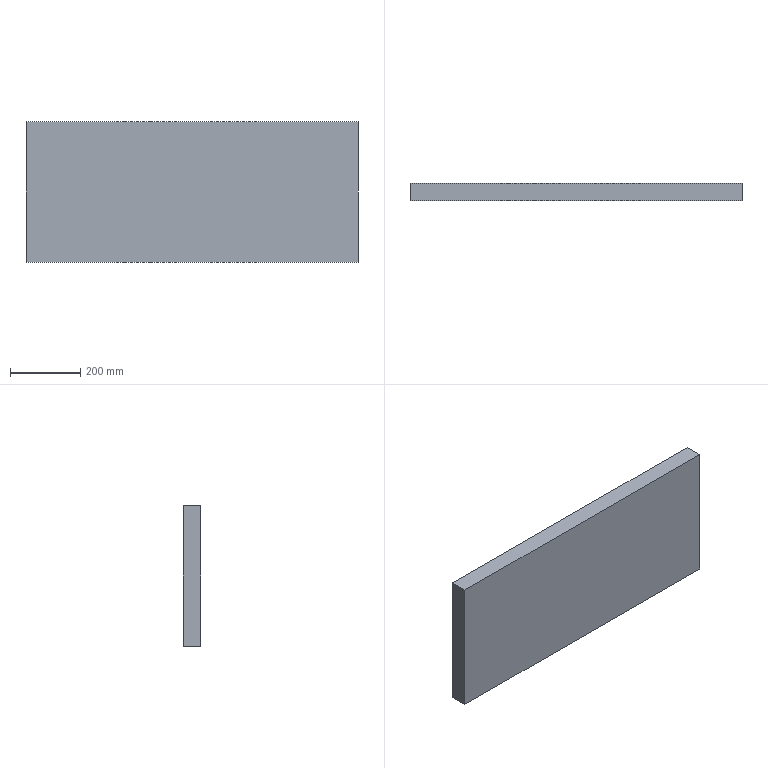Part | STEP file | 1 solid | 6 faces | box 947.9 x 50 x 400 mm | volume 18958001 mm3 | plane 6
STEP:
#1=CARTESIAN_POINT('',(0.,0.,0.));
#2=DIRECTION('',(0.,0.,1.));
#3=DIRECTION('',(1.,0.,0.));
#4=AXIS2_PLACEMENT_3D('',#1,#2,#3);
#5=CARTESIAN_POINT('',(-473.95,-190.836,-56.359));
#6=VERTEX_POINT('',#5);
#7=CARTESIAN_POINT('',(-473.95,-190.836,343.641));
#8=VERTEX_POINT('',#7);
#9=CARTESIAN_POINT('',(-473.95,-190.836,-56.359));
#10=DIRECTION('',(0.,0.,1.));
#11=VECTOR('',#10,1.);
#12=LINE('',#9,#11);
#13=CARTESIAN_POINT('',(-473.95,-240.836,-56.359));
#14=DIRECTION('',(-1.,0.,0.));
#15=DIRECTION('',(0.,-1.,0.));
#16=AXIS2_PLACEMENT_3D('',#13,#14,#15);
#17=PLANE('',#16);
#18=CARTESIAN_POINT('',(-50.,0.));
#19=DIRECTION('',(0.,1.));
#20=VECTOR('',#19,1.);
#21=LINE('',#18,#20);
#22=(GEOMETRIC_REPRESENTATION_CONTEXT(2)PARAMETRIC_REPRESENTATION_CONTEXT()REPRESENTATION_CONTEXT('',''));
#23=DEFINITIONAL_REPRESENTATION('',(#21),#22);
#24=PCURVE('',#17,#23);
#25=CARTESIAN_POINT('',(0.,-190.836,143.641));
#26=DIRECTION('',(0.,1.,0.));
#27=DIRECTION('',(-1.,0.,0.));
#28=AXIS2_PLACEMENT_3D('',#25,#26,#27);
#29=PLANE('',#28);
#30=CARTESIAN_POINT('',(473.95,-200.));
#31=DIRECTION('',(0.,1.));
#32=VECTOR('',#31,1.);
#33=LINE('',#30,#32);
#34=(GEOMETRIC_REPRESENTATION_CONTEXT(2)PARAMETRIC_REPRESENTATION_CONTEXT()REPRESENTATION_CONTEXT('',''));
#35=DEFINITIONAL_REPRESENTATION('',(#33),#34);
#36=PCURVE('',#29,#35);
#37=SURFACE_CURVE('',#12,(#24,#36),.PCURVE_S1.);
#38=EDGE_CURVE('',#6,#8,#37,.T.);
#39=ORIENTED_EDGE('',*,*,#38,.F.);
#40=CARTESIAN_POINT('',(-473.95,-240.836,-56.359));
#41=VERTEX_POINT('',#40);
#42=CARTESIAN_POINT('',(-473.95,-240.836,-56.359));
#43=DIRECTION('',(0.,1.,0.));
#44=VECTOR('',#43,1.);
#45=LINE('',#42,#44);
#46=CARTESIAN_POINT('',(0.,0.));
#47=DIRECTION('',(-1.,0.));
#48=VECTOR('',#47,1.);
#49=LINE('',#46,#48);
#50=(GEOMETRIC_REPRESENTATION_CONTEXT(2)PARAMETRIC_REPRESENTATION_CONTEXT()REPRESENTATION_CONTEXT('',''));
#51=DEFINITIONAL_REPRESENTATION('',(#49),#50);
#52=PCURVE('',#17,#51);
#53=CARTESIAN_POINT('',(-473.95,-240.836,-56.359));
#54=DIRECTION('',(0.,0.,-1.));
#55=DIRECTION('',(-1.,0.,0.));
#56=AXIS2_PLACEMENT_3D('',#53,#54,#55);
#57=PLANE('',#56);
#58=CARTESIAN_POINT('',(0.,0.));
#59=DIRECTION('',(0.,1.));
#60=VECTOR('',#59,1.);
#61=LINE('',#58,#60);
#62=(GEOMETRIC_REPRESENTATION_CONTEXT(2)PARAMETRIC_REPRESENTATION_CONTEXT()REPRESENTATION_CONTEXT('',''));
#63=DEFINITIONAL_REPRESENTATION('',(#61),#62);
#64=PCURVE('',#57,#63);
#65=SURFACE_CURVE('',#45,(#52,#64),.PCURVE_S1.);
#66=EDGE_CURVE('',#41,#6,#65,.T.);
#67=ORIENTED_EDGE('',*,*,#66,.F.);
#68=CARTESIAN_POINT('',(-473.95,-240.836,343.641));
#69=VERTEX_POINT('',#68);
#70=CARTESIAN_POINT('',(-473.95,-240.836,-56.359));
#71=DIRECTION('',(0.,0.,1.));
#72=VECTOR('',#71,1.);
#73=LINE('',#70,#72);
#74=CARTESIAN_POINT('',(0.,0.));
#75=DIRECTION('',(0.,1.));
#76=VECTOR('',#75,1.);
#77=LINE('',#74,#76);
#78=(GEOMETRIC_REPRESENTATION_CONTEXT(2)PARAMETRIC_REPRESENTATION_CONTEXT()REPRESENTATION_CONTEXT('',''));
#79=DEFINITIONAL_REPRESENTATION('',(#77),#78);
#80=PCURVE('',#17,#79);
#81=CARTESIAN_POINT('',(0.,-240.836,143.641));
#82=DIRECTION('',(0.,1.,0.));
#83=DIRECTION('',(-1.,0.,0.));
#84=AXIS2_PLACEMENT_3D('',#81,#82,#83);
#85=PLANE('',#84);
#86=CARTESIAN_POINT('',(473.95,-200.));
#87=DIRECTION('',(0.,1.));
#88=VECTOR('',#87,1.);
#89=LINE('',#86,#88);
#90=(GEOMETRIC_REPRESENTATION_CONTEXT(2)PARAMETRIC_REPRESENTATION_CONTEXT()REPRESENTATION_CONTEXT('',''));
#91=DEFINITIONAL_REPRESENTATION('',(#89),#90);
#92=PCURVE('',#85,#91);
#93=SURFACE_CURVE('',#73,(#80,#92),.PCURVE_S1.);
#94=EDGE_CURVE('',#41,#69,#93,.T.);
#95=ORIENTED_EDGE('',*,*,#94,.T.);
#96=CARTESIAN_POINT('',(-473.95,-240.836,343.641));
#97=DIRECTION('',(0.,1.,0.));
#98=VECTOR('',#97,1.);
#99=LINE('',#96,#98);
#100=CARTESIAN_POINT('',(0.,400.));
#101=DIRECTION('',(-1.,0.));
#102=VECTOR('',#101,1.);
#103=LINE('',#100,#102);
#104=(GEOMETRIC_REPRESENTATION_CONTEXT(2)PARAMETRIC_REPRESENTATION_CONTEXT()REPRESENTATION_CONTEXT('',''));
#105=DEFINITIONAL_REPRESENTATION('',(#103),#104);
#106=PCURVE('',#17,#105);
#107=CARTESIAN_POINT('',(-473.95,-240.836,343.641));
#108=DIRECTION('',(0.,0.,1.));
#109=DIRECTION('',(1.,0.,0.));
#110=AXIS2_PLACEMENT_3D('',#107,#108,#109);
#111=PLANE('',#110);
#112=CARTESIAN_POINT('',(0.,0.));
#113=DIRECTION('',(0.,1.));
#114=VECTOR('',#113,1.);
#115=LINE('',#112,#114);
#116=(GEOMETRIC_REPRESENTATION_CONTEXT(2)PARAMETRIC_REPRESENTATION_CONTEXT()REPRESENTATION_CONTEXT('',''));
#117=DEFINITIONAL_REPRESENTATION('',(#115),#116);
#118=PCURVE('',#111,#117);
#119=SURFACE_CURVE('',#99,(#106,#118),.PCURVE_S1.);
#120=EDGE_CURVE('',#69,#8,#119,.T.);
#121=ORIENTED_EDGE('',*,*,#120,.T.);
#122=EDGE_LOOP('',(#39,#67,#95,#121));
#123=FACE_BOUND('',#122,.T.);
#124=ADVANCED_FACE('',(#123),#17,.T.);
#125=CARTESIAN_POINT('',(473.95,-190.836,-56.359));
#126=VERTEX_POINT('',#125);
#127=CARTESIAN_POINT('',(-473.95,-190.836,-56.359));
#128=DIRECTION('',(-1.,0.,0.));
#129=VECTOR('',#128,1.);
#130=LINE('',#127,#129);
#131=CARTESIAN_POINT('',(0.,50.));
#132=DIRECTION('',(1.,0.));
#133=VECTOR('',#132,1.);
#134=LINE('',#131,#133);
#135=(GEOMETRIC_REPRESENTATION_CONTEXT(2)PARAMETRIC_REPRESENTATION_CONTEXT()REPRESENTATION_CONTEXT('',''));
#136=DEFINITIONAL_REPRESENTATION('',(#134),#135);
#137=PCURVE('',#57,#136);
#138=CARTESIAN_POINT('',(473.95,-200.));
#139=DIRECTION('',(1.,0.));
#140=VECTOR('',#139,1.);
#141=LINE('',#138,#140);
#142=(GEOMETRIC_REPRESENTATION_CONTEXT(2)PARAMETRIC_REPRESENTATION_CONTEXT()REPRESENTATION_CONTEXT('',''));
#143=DEFINITIONAL_REPRESENTATION('',(#141),#142);
#144=PCURVE('',#29,#143);
#145=SURFACE_CURVE('',#130,(#137,#144),.PCURVE_S1.);
#146=EDGE_CURVE('',#126,#6,#145,.T.);
#147=ORIENTED_EDGE('',*,*,#146,.F.);
#148=CARTESIAN_POINT('',(473.95,-240.836,-56.359));
#149=VERTEX_POINT('',#148);
#150=CARTESIAN_POINT('',(473.95,-240.836,-56.359));
#151=DIRECTION('',(0.,1.,0.));
#152=VECTOR('',#151,1.);
#153=LINE('',#150,#152);
#154=CARTESIAN_POINT('',(-947.9,0.));
#155=DIRECTION('',(0.,1.));
#156=VECTOR('',#155,1.);
#157=LINE('',#154,#156);
#158=(GEOMETRIC_REPRESENTATION_CONTEXT(2)PARAMETRIC_REPRESENTATION_CONTEXT()REPRESENTATION_CONTEXT('',''));
#159=DEFINITIONAL_REPRESENTATION('',(#157),#158);
#160=PCURVE('',#57,#159);
#161=CARTESIAN_POINT('',(473.95,-240.836,-56.359));
#162=DIRECTION('',(1.,0.,0.));
#163=DIRECTION('',(0.,1.,0.));
#164=AXIS2_PLACEMENT_3D('',#161,#162,#163);
#165=PLANE('',#164);
#166=CARTESIAN_POINT('',(0.,0.));
#167=DIRECTION('',(1.,0.));
#168=VECTOR('',#167,1.);
#169=LINE('',#166,#168);
#170=(GEOMETRIC_REPRESENTATION_CONTEXT(2)PARAMETRIC_REPRESENTATION_CONTEXT()REPRESENTATION_CONTEXT('',''));
#171=DEFINITIONAL_REPRESENTATION('',(#169),#170);
#172=PCURVE('',#165,#171);
#173=SURFACE_CURVE('',#153,(#160,#172),.PCURVE_S1.);
#174=EDGE_CURVE('',#149,#126,#173,.T.);
#175=ORIENTED_EDGE('',*,*,#174,.F.);
#176=CARTESIAN_POINT('',(-473.95,-240.836,-56.359));
#177=DIRECTION('',(-1.,0.,0.));
#178=VECTOR('',#177,1.);
#179=LINE('',#176,#178);
#180=CARTESIAN_POINT('',(0.,0.));
#181=DIRECTION('',(1.,0.));
#182=VECTOR('',#181,1.);
#183=LINE('',#180,#182);
#184=(GEOMETRIC_REPRESENTATION_CONTEXT(2)PARAMETRIC_REPRESENTATION_CONTEXT()REPRESENTATION_CONTEXT('',''));
#185=DEFINITIONAL_REPRESENTATION('',(#183),#184);
#186=PCURVE('',#57,#185);
#187=CARTESIAN_POINT('',(473.95,-200.));
#188=DIRECTION('',(1.,0.));
#189=VECTOR('',#188,1.);
#190=LINE('',#187,#189);
#191=(GEOMETRIC_REPRESENTATION_CONTEXT(2)PARAMETRIC_REPRESENTATION_CONTEXT()REPRESENTATION_CONTEXT('',''));
#192=DEFINITIONAL_REPRESENTATION('',(#190),#191);
#193=PCURVE('',#85,#192);
#194=SURFACE_CURVE('',#179,(#186,#193),.PCURVE_S1.);
#195=EDGE_CURVE('',#149,#41,#194,.T.);
#196=ORIENTED_EDGE('',*,*,#195,.T.);
#197=ORIENTED_EDGE('',*,*,#66,.T.);
#198=EDGE_LOOP('',(#147,#175,#196,#197));
#199=FACE_BOUND('',#198,.T.);
#200=ADVANCED_FACE('',(#199),#57,.T.);
#201=CARTESIAN_POINT('',(473.95,-190.836,343.641));
#202=VERTEX_POINT('',#201);
#203=CARTESIAN_POINT('',(473.95,-190.836,-56.359));
#204=DIRECTION('',(0.,0.,-1.));
#205=VECTOR('',#204,1.);
#206=LINE('',#203,#205);
#207=CARTESIAN_POINT('',(50.,0.));
#208=DIRECTION('',(0.,-1.));
#209=VECTOR('',#208,1.);
#210=LINE('',#207,#209);
#211=(GEOMETRIC_REPRESENTATION_CONTEXT(2)PARAMETRIC_REPRESENTATION_CONTEXT()REPRESENTATION_CONTEXT('',''));
#212=DEFINITIONAL_REPRESENTATION('',(#210),#211);
#213=PCURVE('',#165,#212);
#214=CARTESIAN_POINT('',(-473.95,-200.));
#215=DIRECTION('',(0.,-1.));
#216=VECTOR('',#215,1.);
#217=LINE('',#214,#216);
#218=(GEOMETRIC_REPRESENTATION_CONTEXT(2)PARAMETRIC_REPRESENTATION_CONTEXT()REPRESENTATION_CONTEXT('',''));
#219=DEFINITIONAL_REPRESENTATION('',(#217),#218);
#220=PCURVE('',#29,#219);
#221=SURFACE_CURVE('',#206,(#213,#220),.PCURVE_S1.);
#222=EDGE_CURVE('',#202,#126,#221,.T.);
#223=ORIENTED_EDGE('',*,*,#222,.F.);
#224=CARTESIAN_POINT('',(473.95,-240.836,343.641));
#225=VERTEX_POINT('',#224);
#226=CARTESIAN_POINT('',(473.95,-240.836,343.641));
#227=DIRECTION('',(0.,1.,0.));
#228=VECTOR('',#227,1.);
#229=LINE('',#226,#228);
#230=CARTESIAN_POINT('',(0.,400.));
#231=DIRECTION('',(1.,0.));
#232=VECTOR('',#231,1.);
#233=LINE('',#230,#232);
#234=(GEOMETRIC_REPRESENTATION_CONTEXT(2)PARAMETRIC_REPRESENTATION_CONTEXT()REPRESENTATION_CONTEXT('',''));
#235=DEFINITIONAL_REPRESENTATION('',(#233),#234);
#236=PCURVE('',#165,#235);
#237=CARTESIAN_POINT('',(947.9,0.));
#238=DIRECTION('',(0.,1.));
#239=VECTOR('',#238,1.);
#240=LINE('',#237,#239);
#241=(GEOMETRIC_REPRESENTATION_CONTEXT(2)PARAMETRIC_REPRESENTATION_CONTEXT()REPRESENTATION_CONTEXT('',''));
#242=DEFINITIONAL_REPRESENTATION('',(#240),#241);
#243=PCURVE('',#111,#242);
#244=SURFACE_CURVE('',#229,(#236,#243),.PCURVE_S1.);
#245=EDGE_CURVE('',#225,#202,#244,.T.);
#246=ORIENTED_EDGE('',*,*,#245,.F.);
#247=CARTESIAN_POINT('',(473.95,-240.836,-56.359));
#248=DIRECTION('',(0.,0.,-1.));
#249=VECTOR('',#248,1.);
#250=LINE('',#247,#249);
#251=CARTESIAN_POINT('',(0.,0.));
#252=DIRECTION('',(0.,-1.));
#253=VECTOR('',#252,1.);
#254=LINE('',#251,#253);
#255=(GEOMETRIC_REPRESENTATION_CONTEXT(2)PARAMETRIC_REPRESENTATION_CONTEXT()REPRESENTATION_CONTEXT('',''));
#256=DEFINITIONAL_REPRESENTATION('',(#254),#255);
#257=PCURVE('',#165,#256);
#258=CARTESIAN_POINT('',(-473.95,-200.));
#259=DIRECTION('',(0.,-1.));
#260=VECTOR('',#259,1.);
#261=LINE('',#258,#260);
#262=(GEOMETRIC_REPRESENTATION_CONTEXT(2)PARAMETRIC_REPRESENTATION_CONTEXT()REPRESENTATION_CONTEXT('',''));
#263=DEFINITIONAL_REPRESENTATION('',(#261),#262);
#264=PCURVE('',#85,#263);
#265=SURFACE_CURVE('',#250,(#257,#264),.PCURVE_S1.);
#266=EDGE_CURVE('',#225,#149,#265,.T.);
#267=ORIENTED_EDGE('',*,*,#266,.T.);
#268=ORIENTED_EDGE('',*,*,#174,.T.);
#269=EDGE_LOOP('',(#223,#246,#267,#268));
#270=FACE_BOUND('',#269,.T.);
#271=ADVANCED_FACE('',(#270),#165,.T.);
#272=CARTESIAN_POINT('',(-473.95,-190.836,343.641));
#273=DIRECTION('',(1.,0.,0.));
#274=VECTOR('',#273,1.);
#275=LINE('',#272,#274);
#276=CARTESIAN_POINT('',(0.,50.));
#277=DIRECTION('',(1.,0.));
#278=VECTOR('',#277,1.);
#279=LINE('',#276,#278);
#280=(GEOMETRIC_REPRESENTATION_CONTEXT(2)PARAMETRIC_REPRESENTATION_CONTEXT()REPRESENTATION_CONTEXT('',''));
#281=DEFINITIONAL_REPRESENTATION('',(#279),#280);
#282=PCURVE('',#111,#281);
#283=CARTESIAN_POINT('',(473.95,200.));
#284=DIRECTION('',(-1.,0.));
#285=VECTOR('',#284,1.);
#286=LINE('',#283,#285);
#287=(GEOMETRIC_REPRESENTATION_CONTEXT(2)PARAMETRIC_REPRESENTATION_CONTEXT()REPRESENTATION_CONTEXT('',''));
#288=DEFINITIONAL_REPRESENTATION('',(#286),#287);
#289=PCURVE('',#29,#288);
#290=SURFACE_CURVE('',#275,(#282,#289),.PCURVE_S1.);
#291=EDGE_CURVE('',#8,#202,#290,.T.);
#292=ORIENTED_EDGE('',*,*,#291,.F.);
#293=ORIENTED_EDGE('',*,*,#120,.F.);
#294=CARTESIAN_POINT('',(-473.95,-240.836,343.641));
#295=DIRECTION('',(1.,0.,0.));
#296=VECTOR('',#295,1.);
#297=LINE('',#294,#296);
#298=CARTESIAN_POINT('',(0.,0.));
#299=DIRECTION('',(1.,0.));
#300=VECTOR('',#299,1.);
#301=LINE('',#298,#300);
#302=(GEOMETRIC_REPRESENTATION_CONTEXT(2)PARAMETRIC_REPRESENTATION_CONTEXT()REPRESENTATION_CONTEXT('',''));
#303=DEFINITIONAL_REPRESENTATION('',(#301),#302);
#304=PCURVE('',#111,#303);
#305=CARTESIAN_POINT('',(473.95,200.));
#306=DIRECTION('',(-1.,0.));
#307=VECTOR('',#306,1.);
#308=LINE('',#305,#307);
#309=(GEOMETRIC_REPRESENTATION_CONTEXT(2)PARAMETRIC_REPRESENTATION_CONTEXT()REPRESENTATION_CONTEXT('',''));
#310=DEFINITIONAL_REPRESENTATION('',(#308),#309);
#311=PCURVE('',#85,#310);
#312=SURFACE_CURVE('',#297,(#304,#311),.PCURVE_S1.);
#313=EDGE_CURVE('',#69,#225,#312,.T.);
#314=ORIENTED_EDGE('',*,*,#313,.T.);
#315=ORIENTED_EDGE('',*,*,#245,.T.);
#316=EDGE_LOOP('',(#292,#293,#314,#315));
#317=FACE_BOUND('',#316,.T.);
#318=ADVANCED_FACE('',(#317),#111,.T.);
#319=ORIENTED_EDGE('',*,*,#94,.F.);
#320=ORIENTED_EDGE('',*,*,#195,.F.);
#321=ORIENTED_EDGE('',*,*,#266,.F.);
#322=ORIENTED_EDGE('',*,*,#313,.F.);
#323=EDGE_LOOP('',(#319,#320,#321,#322));
#324=FACE_BOUND('',#323,.T.);
#325=ADVANCED_FACE('',(#324),#85,.F.);
#326=ORIENTED_EDGE('',*,*,#38,.T.);
#327=ORIENTED_EDGE('',*,*,#291,.T.);
#328=ORIENTED_EDGE('',*,*,#222,.T.);
#329=ORIENTED_EDGE('',*,*,#146,.T.);
#330=EDGE_LOOP('',(#326,#327,#328,#329));
#331=FACE_BOUND('',#330,.T.);
#332=ADVANCED_FACE('',(#331),#29,.T.);
#333=CLOSED_SHELL('',(#124,#200,#271,#318,#325,#332));
#334=MANIFOLD_SOLID_BREP('',#333);
#335=(LENGTH_UNIT()NAMED_UNIT(*)SI_UNIT(.MILLI.,.METRE.));
#336=UNCERTAINTY_MEASURE_WITH_UNIT(LENGTH_MEASURE(0.0000001),#335,'','');
#337=(NAMED_UNIT(*)PLANE_ANGLE_UNIT()SI_UNIT($,.RADIAN.));
#338=(NAMED_UNIT(*)SI_UNIT($,.STERADIAN.)SOLID_ANGLE_UNIT());
#339=(GEOMETRIC_REPRESENTATION_CONTEXT(3)GLOBAL_UNCERTAINTY_ASSIGNED_CONTEXT((#336))GLOBAL_UNIT_ASSIGNED_CONTEXT((#335,#337,#338))REPRESENTATION_CONTEXT('',''));
#340=ADVANCED_BREP_SHAPE_REPRESENTATION('',(#4,#334),#339);